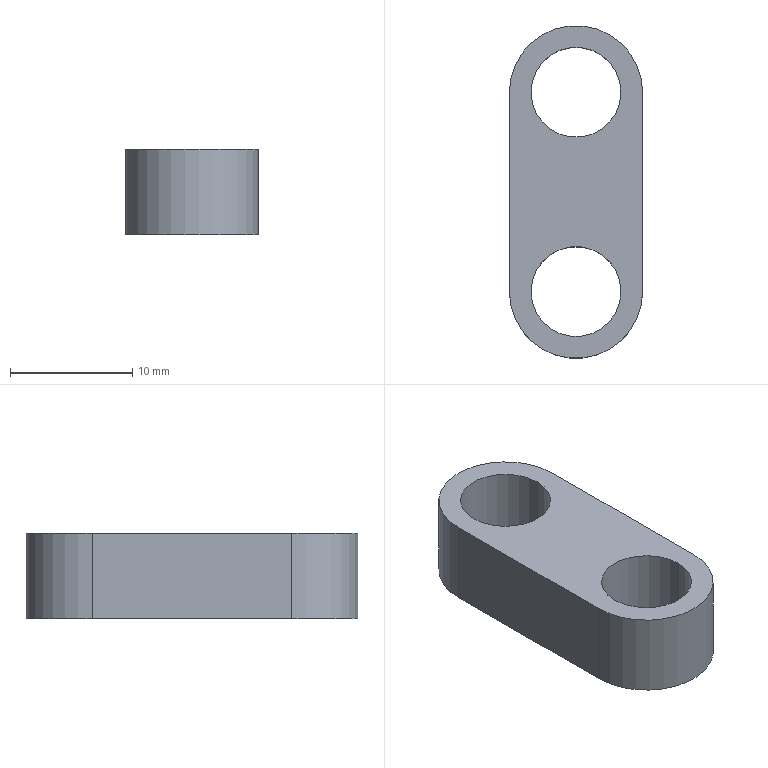Part | SolidWorks | features Cut 2, Extrusion 1 | 1 solid | 10 faces | box 10.89 x 27.179 x 7 mm | volume 1300 mm3 | cylinder 6 | plane 4 | commonest cylinder face diameters 7.349 x4 10.89 x2
STEP:
#1=CARTESIAN_POINT('',(-30.74,16.289,-3.5));
#2=VERTEX_POINT('',#1);
#3=CARTESIAN_POINT('',(-23.391,16.289,-3.5));
#4=VERTEX_POINT('',#3);
#5=CARTESIAN_POINT('',(-27.066,16.289,-3.5));
#6=DIRECTION('',(0.,0.,1.));
#7=DIRECTION('',(1.,0.,0.));
#8=AXIS2_PLACEMENT_3D('',#5,#6,#7);
#9=CIRCLE('',#8,3.675);
#10=EDGE_CURVE('',#2,#4,#9,.T.);
#11=ORIENTED_EDGE('',*,*,#10,.F.);
#12=CARTESIAN_POINT('',(-30.74,16.289,3.5));
#13=VERTEX_POINT('',#12);
#14=CARTESIAN_POINT('',(-30.74,16.289,-6.5));
#15=DIRECTION('',(0.,0.,1.));
#16=VECTOR('',#15,1000.);
#17=LINE('',#14,#16);
#18=EDGE_CURVE('',#2,#13,#17,.T.);
#19=ORIENTED_EDGE('',*,*,#18,.T.);
#20=CARTESIAN_POINT('',(-23.391,16.289,3.5));
#21=VERTEX_POINT('',#20);
#22=CARTESIAN_POINT('',(-27.066,16.289,3.5));
#23=DIRECTION('',(0.,0.,1.));
#24=DIRECTION('',(1.,0.,0.));
#25=AXIS2_PLACEMENT_3D('',#22,#23,#24);
#26=CIRCLE('',#25,3.675);
#27=EDGE_CURVE('',#13,#21,#26,.T.);
#28=ORIENTED_EDGE('',*,*,#27,.T.);
#29=CARTESIAN_POINT('',(-23.391,16.289,-6.5));
#30=DIRECTION('',(0.,0.,1.));
#31=VECTOR('',#30,1000.);
#32=LINE('',#29,#31);
#33=EDGE_CURVE('',#4,#21,#32,.T.);
#34=ORIENTED_EDGE('',*,*,#33,.F.);
#35=EDGE_LOOP('',(#11,#19,#28,#34));
#36=FACE_OUTER_BOUND('',#35,.T.);
#37=CARTESIAN_POINT('',(-27.066,16.289,-6.5));
#38=DIRECTION('',(0.,0.,1.));
#39=DIRECTION('',(1.,0.,0.));
#40=AXIS2_PLACEMENT_3D('',#37,#38,#39);
#41=CYLINDRICAL_SURFACE('',#40,3.675);
#42=ADVANCED_FACE('',(#36),#41,.F.);
#43=CARTESIAN_POINT('',(-30.74,0.,-3.5));
#44=VERTEX_POINT('',#43);
#45=CARTESIAN_POINT('',(-23.391,0.,-3.5));
#46=VERTEX_POINT('',#45);
#47=CARTESIAN_POINT('',(-27.066,0.,-3.5));
#48=DIRECTION('',(0.,0.,1.));
#49=DIRECTION('',(1.,0.,0.));
#50=AXIS2_PLACEMENT_3D('',#47,#48,#49);
#51=CIRCLE('',#50,3.675);
#52=EDGE_CURVE('',#44,#46,#51,.T.);
#53=ORIENTED_EDGE('',*,*,#52,.F.);
#54=CARTESIAN_POINT('',(-30.74,0.,3.5));
#55=VERTEX_POINT('',#54);
#56=CARTESIAN_POINT('',(-30.74,0.,-6.5));
#57=DIRECTION('',(0.,0.,1.));
#58=VECTOR('',#57,1000.);
#59=LINE('',#56,#58);
#60=EDGE_CURVE('',#44,#55,#59,.T.);
#61=ORIENTED_EDGE('',*,*,#60,.T.);
#62=CARTESIAN_POINT('',(-23.391,0.,3.5));
#63=VERTEX_POINT('',#62);
#64=CARTESIAN_POINT('',(-27.066,0.,3.5));
#65=DIRECTION('',(0.,0.,1.));
#66=DIRECTION('',(1.,0.,0.));
#67=AXIS2_PLACEMENT_3D('',#64,#65,#66);
#68=CIRCLE('',#67,3.675);
#69=EDGE_CURVE('',#55,#63,#68,.T.);
#70=ORIENTED_EDGE('',*,*,#69,.T.);
#71=CARTESIAN_POINT('',(-23.391,0.,-6.5));
#72=DIRECTION('',(0.,0.,1.));
#73=VECTOR('',#72,1000.);
#74=LINE('',#71,#73);
#75=EDGE_CURVE('',#46,#63,#74,.T.);
#76=ORIENTED_EDGE('',*,*,#75,.F.);
#77=EDGE_LOOP('',(#53,#61,#70,#76));
#78=FACE_OUTER_BOUND('',#77,.T.);
#79=CARTESIAN_POINT('',(-27.066,0.,-6.5));
#80=DIRECTION('',(0.,0.,1.));
#81=DIRECTION('',(1.,0.,0.));
#82=AXIS2_PLACEMENT_3D('',#79,#80,#81);
#83=CYLINDRICAL_SURFACE('',#82,3.675);
#84=ADVANCED_FACE('',(#78),#83,.F.);
#85=CARTESIAN_POINT('',(-21.621,16.289,-3.5));
#86=VERTEX_POINT('',#85);
#87=CARTESIAN_POINT('',(-32.511,16.289,-3.5));
#88=VERTEX_POINT('',#87);
#89=CARTESIAN_POINT('',(-27.066,16.289,-3.5));
#90=DIRECTION('',(0.,0.,1.));
#91=DIRECTION('',(1.,0.,0.));
#92=AXIS2_PLACEMENT_3D('',#89,#90,#91);
#93=CIRCLE('',#92,5.445);
#94=EDGE_CURVE('',#86,#88,#93,.T.);
#95=ORIENTED_EDGE('',*,*,#94,.T.);
#96=CARTESIAN_POINT('',(-32.511,16.289,3.5));
#97=VERTEX_POINT('',#96);
#98=CARTESIAN_POINT('',(-32.511,16.289,3.5));
#99=DIRECTION('',(0.,0.,-1.));
#100=VECTOR('',#99,1000.);
#101=LINE('',#98,#100);
#102=EDGE_CURVE('',#97,#88,#101,.T.);
#103=ORIENTED_EDGE('',*,*,#102,.F.);
#104=CARTESIAN_POINT('',(-21.621,16.289,3.5));
#105=VERTEX_POINT('',#104);
#106=CARTESIAN_POINT('',(-27.066,16.289,3.5));
#107=DIRECTION('',(0.,0.,1.));
#108=DIRECTION('',(1.,0.,0.));
#109=AXIS2_PLACEMENT_3D('',#106,#107,#108);
#110=CIRCLE('',#109,5.445);
#111=EDGE_CURVE('',#105,#97,#110,.T.);
#112=ORIENTED_EDGE('',*,*,#111,.F.);
#113=CARTESIAN_POINT('',(-21.621,16.289,3.5));
#114=DIRECTION('',(0.,0.,-1.));
#115=VECTOR('',#114,1000.);
#116=LINE('',#113,#115);
#117=EDGE_CURVE('',#105,#86,#116,.T.);
#118=ORIENTED_EDGE('',*,*,#117,.T.);
#119=EDGE_LOOP('',(#95,#103,#112,#118));
#120=FACE_OUTER_BOUND('',#119,.T.);
#121=CARTESIAN_POINT('',(-27.066,16.289,3.5));
#122=DIRECTION('',(0.,0.,-1.));
#123=DIRECTION('',(-1.,0.,0.));
#124=AXIS2_PLACEMENT_3D('',#121,#122,#123);
#125=CYLINDRICAL_SURFACE('',#124,5.445);
#126=ADVANCED_FACE('',(#120),#125,.T.);
#127=CARTESIAN_POINT('',(-32.511,0.,-3.5));
#128=VERTEX_POINT('',#127);
#129=CARTESIAN_POINT('',(-32.511,16.289,-3.5));
#130=DIRECTION('',(0.,-1.,0.));
#131=VECTOR('',#130,1000.);
#132=LINE('',#129,#131);
#133=EDGE_CURVE('',#88,#128,#132,.T.);
#134=ORIENTED_EDGE('',*,*,#133,.T.);
#135=CARTESIAN_POINT('',(-32.511,0.,3.5));
#136=VERTEX_POINT('',#135);
#137=CARTESIAN_POINT('',(-32.511,0.,3.5));
#138=DIRECTION('',(0.,0.,-1.));
#139=VECTOR('',#138,1000.);
#140=LINE('',#137,#139);
#141=EDGE_CURVE('',#136,#128,#140,.T.);
#142=ORIENTED_EDGE('',*,*,#141,.F.);
#143=CARTESIAN_POINT('',(-32.511,16.289,3.5));
#144=DIRECTION('',(0.,-1.,0.));
#145=VECTOR('',#144,1000.);
#146=LINE('',#143,#145);
#147=EDGE_CURVE('',#97,#136,#146,.T.);
#148=ORIENTED_EDGE('',*,*,#147,.F.);
#149=ORIENTED_EDGE('',*,*,#102,.T.);
#150=EDGE_LOOP('',(#134,#142,#148,#149));
#151=FACE_OUTER_BOUND('',#150,.T.);
#152=CARTESIAN_POINT('',(-32.511,16.289,3.5));
#153=DIRECTION('',(1.,0.,0.));
#154=DIRECTION('',(0.,0.,-1.));
#155=AXIS2_PLACEMENT_3D('',#152,#153,#154);
#156=PLANE('',#155);
#157=ADVANCED_FACE('',(#151),#156,.F.);
#158=CARTESIAN_POINT('',(-21.621,0.,-3.5));
#159=VERTEX_POINT('',#158);
#160=CARTESIAN_POINT('',(-27.066,0.,-3.5));
#161=DIRECTION('',(0.,0.,1.));
#162=DIRECTION('',(1.,0.,0.));
#163=AXIS2_PLACEMENT_3D('',#160,#161,#162);
#164=CIRCLE('',#163,5.445);
#165=EDGE_CURVE('',#128,#159,#164,.T.);
#166=ORIENTED_EDGE('',*,*,#165,.T.);
#167=CARTESIAN_POINT('',(-21.621,0.,3.5));
#168=VERTEX_POINT('',#167);
#169=CARTESIAN_POINT('',(-21.621,0.,3.5));
#170=DIRECTION('',(0.,0.,-1.));
#171=VECTOR('',#170,1000.);
#172=LINE('',#169,#171);
#173=EDGE_CURVE('',#168,#159,#172,.T.);
#174=ORIENTED_EDGE('',*,*,#173,.F.);
#175=CARTESIAN_POINT('',(-27.066,0.,3.5));
#176=DIRECTION('',(0.,0.,1.));
#177=DIRECTION('',(1.,0.,0.));
#178=AXIS2_PLACEMENT_3D('',#175,#176,#177);
#179=CIRCLE('',#178,5.445);
#180=EDGE_CURVE('',#136,#168,#179,.T.);
#181=ORIENTED_EDGE('',*,*,#180,.F.);
#182=ORIENTED_EDGE('',*,*,#141,.T.);
#183=EDGE_LOOP('',(#166,#174,#181,#182));
#184=FACE_OUTER_BOUND('',#183,.T.);
#185=CARTESIAN_POINT('',(-27.066,0.,3.5));
#186=DIRECTION('',(0.,0.,-1.));
#187=DIRECTION('',(-1.,0.,0.));
#188=AXIS2_PLACEMENT_3D('',#185,#186,#187);
#189=CYLINDRICAL_SURFACE('',#188,5.445);
#190=ADVANCED_FACE('',(#184),#189,.T.);
#191=CARTESIAN_POINT('',(-21.621,16.289,-3.5));
#192=DIRECTION('',(0.,-1.,0.));
#193=VECTOR('',#192,1000.);
#194=LINE('',#191,#193);
#195=EDGE_CURVE('',#86,#159,#194,.T.);
#196=ORIENTED_EDGE('',*,*,#195,.F.);
#197=ORIENTED_EDGE('',*,*,#117,.F.);
#198=CARTESIAN_POINT('',(-21.621,16.289,3.5));
#199=DIRECTION('',(0.,-1.,0.));
#200=VECTOR('',#199,1000.);
#201=LINE('',#198,#200);
#202=EDGE_CURVE('',#105,#168,#201,.T.);
#203=ORIENTED_EDGE('',*,*,#202,.T.);
#204=ORIENTED_EDGE('',*,*,#173,.T.);
#205=EDGE_LOOP('',(#196,#197,#203,#204));
#206=FACE_OUTER_BOUND('',#205,.T.);
#207=CARTESIAN_POINT('',(-21.621,16.289,3.5));
#208=DIRECTION('',(1.,0.,0.));
#209=DIRECTION('',(0.,0.,-1.));
#210=AXIS2_PLACEMENT_3D('',#207,#208,#209);
#211=PLANE('',#210);
#212=ADVANCED_FACE('',(#206),#211,.T.);
#213=CARTESIAN_POINT('',(-27.066,16.289,3.5));
#214=DIRECTION('',(0.,0.,1.));
#215=DIRECTION('',(1.,0.,0.));
#216=AXIS2_PLACEMENT_3D('',#213,#214,#215);
#217=CIRCLE('',#216,3.675);
#218=EDGE_CURVE('',#21,#13,#217,.T.);
#219=ORIENTED_EDGE('',*,*,#218,.F.);
#220=ORIENTED_EDGE('',*,*,#27,.F.);
#221=EDGE_LOOP('',(#219,#220));
#222=FACE_BOUND('',#221,.T.);
#223=CARTESIAN_POINT('',(-27.066,0.,3.5));
#224=DIRECTION('',(0.,0.,1.));
#225=DIRECTION('',(1.,0.,0.));
#226=AXIS2_PLACEMENT_3D('',#223,#224,#225);
#227=CIRCLE('',#226,3.675);
#228=EDGE_CURVE('',#63,#55,#227,.T.);
#229=ORIENTED_EDGE('',*,*,#228,.F.);
#230=ORIENTED_EDGE('',*,*,#69,.F.);
#231=EDGE_LOOP('',(#229,#230));
#232=FACE_BOUND('',#231,.T.);
#233=ORIENTED_EDGE('',*,*,#111,.T.);
#234=ORIENTED_EDGE('',*,*,#147,.T.);
#235=ORIENTED_EDGE('',*,*,#180,.T.);
#236=ORIENTED_EDGE('',*,*,#202,.F.);
#237=EDGE_LOOP('',(#233,#234,#235,#236));
#238=FACE_OUTER_BOUND('',#237,.T.);
#239=CARTESIAN_POINT('',(-27.066,16.289,3.5));
#240=DIRECTION('',(0.,0.,1.));
#241=DIRECTION('',(1.,0.,0.));
#242=AXIS2_PLACEMENT_3D('',#239,#240,#241);
#243=PLANE('',#242);
#244=ADVANCED_FACE('',(#222,#232,#238),#243,.T.);
#245=CARTESIAN_POINT('',(-27.066,16.289,-3.5));
#246=DIRECTION('',(0.,0.,1.));
#247=DIRECTION('',(1.,0.,0.));
#248=AXIS2_PLACEMENT_3D('',#245,#246,#247);
#249=CIRCLE('',#248,3.675);
#250=EDGE_CURVE('',#4,#2,#249,.T.);
#251=ORIENTED_EDGE('',*,*,#250,.T.);
#252=ORIENTED_EDGE('',*,*,#10,.T.);
#253=EDGE_LOOP('',(#251,#252));
#254=FACE_BOUND('',#253,.T.);
#255=CARTESIAN_POINT('',(-27.066,0.,-3.5));
#256=DIRECTION('',(0.,0.,1.));
#257=DIRECTION('',(1.,0.,0.));
#258=AXIS2_PLACEMENT_3D('',#255,#256,#257);
#259=CIRCLE('',#258,3.675);
#260=EDGE_CURVE('',#46,#44,#259,.T.);
#261=ORIENTED_EDGE('',*,*,#260,.T.);
#262=ORIENTED_EDGE('',*,*,#52,.T.);
#263=EDGE_LOOP('',(#261,#262));
#264=FACE_BOUND('',#263,.T.);
#265=ORIENTED_EDGE('',*,*,#94,.F.);
#266=ORIENTED_EDGE('',*,*,#195,.T.);
#267=ORIENTED_EDGE('',*,*,#165,.F.);
#268=ORIENTED_EDGE('',*,*,#133,.F.);
#269=EDGE_LOOP('',(#265,#266,#267,#268));
#270=FACE_OUTER_BOUND('',#269,.T.);
#271=CARTESIAN_POINT('',(-27.066,16.289,-3.5));
#272=DIRECTION('',(0.,0.,1.));
#273=DIRECTION('',(1.,0.,0.));
#274=AXIS2_PLACEMENT_3D('',#271,#272,#273);
#275=PLANE('',#274);
#276=ADVANCED_FACE('',(#254,#264,#270),#275,.F.);
#277=ORIENTED_EDGE('',*,*,#60,.F.);
#278=ORIENTED_EDGE('',*,*,#260,.F.);
#279=ORIENTED_EDGE('',*,*,#75,.T.);
#280=ORIENTED_EDGE('',*,*,#228,.T.);
#281=EDGE_LOOP('',(#277,#278,#279,#280));
#282=FACE_OUTER_BOUND('',#281,.T.);
#283=CARTESIAN_POINT('',(-27.066,0.,-6.5));
#284=DIRECTION('',(0.,0.,1.));
#285=DIRECTION('',(1.,0.,0.));
#286=AXIS2_PLACEMENT_3D('',#283,#284,#285);
#287=CYLINDRICAL_SURFACE('',#286,3.675);
#288=ADVANCED_FACE('',(#282),#287,.F.);
#289=ORIENTED_EDGE('',*,*,#18,.F.);
#290=ORIENTED_EDGE('',*,*,#250,.F.);
#291=ORIENTED_EDGE('',*,*,#33,.T.);
#292=ORIENTED_EDGE('',*,*,#218,.T.);
#293=EDGE_LOOP('',(#289,#290,#291,#292));
#294=FACE_OUTER_BOUND('',#293,.T.);
#295=CARTESIAN_POINT('',(-27.066,16.289,-6.5));
#296=DIRECTION('',(0.,0.,1.));
#297=DIRECTION('',(1.,0.,0.));
#298=AXIS2_PLACEMENT_3D('',#295,#296,#297);
#299=CYLINDRICAL_SURFACE('',#298,3.675);
#300=ADVANCED_FACE('',(#294),#299,.F.);
#301=CLOSED_SHELL('',(#42,#84,#126,#157,#190,#212,#244,#276,#288,#300));
#302=MANIFOLD_SOLID_BREP('',#301);
#303=CARTESIAN_POINT('',(0.,0.,0.));
#304=DIRECTION('',(0.,0.,1.));
#305=DIRECTION('',(1.,0.,0.));
#306=AXIS2_PLACEMENT_3D('',#303,#304,#305);
#307=(LENGTH_UNIT()NAMED_UNIT(*)SI_UNIT(.MILLI.,.METRE.));
#308=UNCERTAINTY_MEASURE_WITH_UNIT(LENGTH_MEASURE(0.00001),#307,'','');
#309=(NAMED_UNIT(*)PLANE_ANGLE_UNIT()SI_UNIT($,.RADIAN.));
#310=(NAMED_UNIT(*)SI_UNIT($,.STERADIAN.)SOLID_ANGLE_UNIT());
#311=(GEOMETRIC_REPRESENTATION_CONTEXT(3)GLOBAL_UNCERTAINTY_ASSIGNED_CONTEXT((#308))GLOBAL_UNIT_ASSIGNED_CONTEXT((#307,#309,#310))REPRESENTATION_CONTEXT('',''));
#312=ADVANCED_BREP_SHAPE_REPRESENTATION('',(#302,#306),#311);